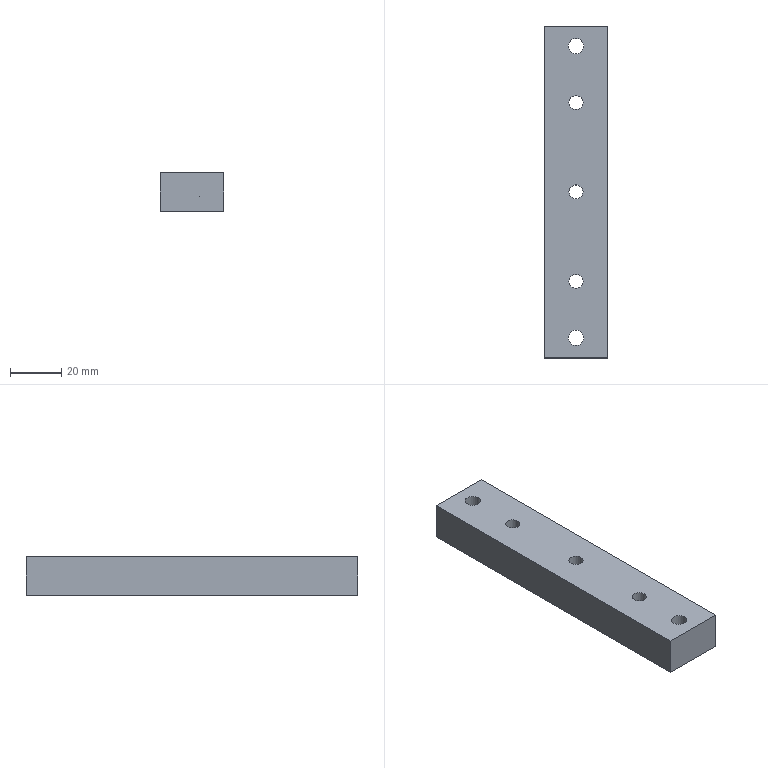Part | STEP file | 200 mesh_id1994 | 1 solid | 11 faces | box 25 x 130 x 15 mm | volume 46833 mm3 | plane 6 | cylinder 5 | commonest cylinder face diameters 5.5 x3 6 x2
STEP:
#1=CARTESIAN_POINT('',(-17225.384,-3957.819,95.));
#2=VERTEX_POINT('',#1);
#3=CARTESIAN_POINT('',(-17225.384,-4087.819,95.));
#4=VERTEX_POINT('',#3);
#5=CARTESIAN_POINT('',(-17225.384,-3961.669,95.));
#6=DIRECTION('',(0.,-1.,0.));
#7=VECTOR('',#6,1.);
#8=LINE('',#5,#7);
#9=EDGE_CURVE('',#2,#4,#8,.T.);
#10=ORIENTED_EDGE('',*,*,#9,.F.);
#11=CARTESIAN_POINT('',(-17225.384,-3957.819,80.));
#12=VERTEX_POINT('',#11);
#13=CARTESIAN_POINT('',(-17225.384,-3957.819,92.));
#14=DIRECTION('',(0.,0.,-1.));
#15=VECTOR('',#14,1.);
#16=LINE('',#13,#15);
#17=EDGE_CURVE('',#2,#12,#16,.T.);
#18=ORIENTED_EDGE('',*,*,#17,.T.);
#19=CARTESIAN_POINT('',(-17225.384,-4087.819,80.));
#20=VERTEX_POINT('',#19);
#21=CARTESIAN_POINT('',(-17225.384,-3961.669,80.));
#22=DIRECTION('',(0.,-1.,0.));
#23=VECTOR('',#22,1.);
#24=LINE('',#21,#23);
#25=EDGE_CURVE('',#12,#20,#24,.T.);
#26=ORIENTED_EDGE('',*,*,#25,.T.);
#27=CARTESIAN_POINT('',(-17225.384,-4087.819,92.));
#28=DIRECTION('',(0.,0.,-1.));
#29=VECTOR('',#28,1.);
#30=LINE('',#27,#29);
#31=EDGE_CURVE('',#4,#20,#30,.T.);
#32=ORIENTED_EDGE('',*,*,#31,.F.);
#33=EDGE_LOOP('',(#10,#18,#26,#32));
#34=FACE_OUTER_BOUND('',#33,.T.);
#35=CARTESIAN_POINT('',(-17225.384,-3961.669,92.));
#36=DIRECTION('',(1.,0.,0.));
#37=DIRECTION('',(0.,0.,1.));
#38=AXIS2_PLACEMENT_3D('',#35,#36,#37);
#39=PLANE('',#38);
#40=ADVANCED_FACE('',(#34),#39,.F.);
#41=CARTESIAN_POINT('',(-17200.384,-4087.819,80.));
#42=VERTEX_POINT('',#41);
#43=CARTESIAN_POINT('',(-17200.384,-3957.819,80.));
#44=VERTEX_POINT('',#43);
#45=CARTESIAN_POINT('',(-17200.384,-4083.969,80.));
#46=DIRECTION('',(0.,1.,0.));
#47=VECTOR('',#46,1.);
#48=LINE('',#45,#47);
#49=EDGE_CURVE('',#42,#44,#48,.T.);
#50=ORIENTED_EDGE('',*,*,#49,.T.);
#51=CARTESIAN_POINT('',(-17200.384,-3957.819,95.));
#52=VERTEX_POINT('',#51);
#53=CARTESIAN_POINT('',(-17200.384,-3957.819,92.));
#54=DIRECTION('',(0.,0.,-1.));
#55=VECTOR('',#54,1.);
#56=LINE('',#53,#55);
#57=EDGE_CURVE('',#52,#44,#56,.T.);
#58=ORIENTED_EDGE('',*,*,#57,.F.);
#59=CARTESIAN_POINT('',(-17200.384,-4087.819,95.));
#60=VERTEX_POINT('',#59);
#61=CARTESIAN_POINT('',(-17200.384,-4083.969,95.));
#62=DIRECTION('',(0.,1.,0.));
#63=VECTOR('',#62,1.);
#64=LINE('',#61,#63);
#65=EDGE_CURVE('',#60,#52,#64,.T.);
#66=ORIENTED_EDGE('',*,*,#65,.F.);
#67=CARTESIAN_POINT('',(-17200.384,-4087.819,92.));
#68=DIRECTION('',(0.,0.,-1.));
#69=VECTOR('',#68,1.);
#70=LINE('',#67,#69);
#71=EDGE_CURVE('',#60,#42,#70,.T.);
#72=ORIENTED_EDGE('',*,*,#71,.T.);
#73=EDGE_LOOP('',(#50,#58,#66,#72));
#74=FACE_OUTER_BOUND('',#73,.T.);
#75=CARTESIAN_POINT('',(-17200.384,-4083.969,92.));
#76=DIRECTION('',(-1.,0.,0.));
#77=DIRECTION('',(0.,0.,-1.));
#78=AXIS2_PLACEMENT_3D('',#75,#76,#77);
#79=PLANE('',#78);
#80=ADVANCED_FACE('',(#74),#79,.F.);
#81=CARTESIAN_POINT('',(-17209.884,-4079.969,95.));
#82=VERTEX_POINT('',#81);
#83=CARTESIAN_POINT('',(-17212.884,-4079.969,95.));
#84=DIRECTION('',(0.,0.,-1.));
#85=DIRECTION('',(1.,0.,0.));
#86=AXIS2_PLACEMENT_3D('',#83,#84,#85);
#87=CIRCLE('',#86,3.);
#88=EDGE_CURVE('',#82,#82,#87,.T.);
#89=ORIENTED_EDGE('',*,*,#88,.T.);
#90=EDGE_LOOP('',(#89));
#91=FACE_BOUND('',#90,.T.);
#92=CARTESIAN_POINT('',(-17209.884,-3965.669,95.));
#93=VERTEX_POINT('',#92);
#94=CARTESIAN_POINT('',(-17212.884,-3965.669,95.));
#95=DIRECTION('',(0.,0.,-1.));
#96=DIRECTION('',(1.,0.,0.));
#97=AXIS2_PLACEMENT_3D('',#94,#95,#96);
#98=CIRCLE('',#97,3.);
#99=EDGE_CURVE('',#93,#93,#98,.T.);
#100=ORIENTED_EDGE('',*,*,#99,.T.);
#101=EDGE_LOOP('',(#100));
#102=FACE_BOUND('',#101,.T.);
#103=ORIENTED_EDGE('',*,*,#65,.T.);
#104=CARTESIAN_POINT('',(-17200.384,-3957.819,95.));
#105=DIRECTION('',(-1.,0.,0.));
#106=VECTOR('',#105,1.);
#107=LINE('',#104,#106);
#108=EDGE_CURVE('',#52,#2,#107,.T.);
#109=ORIENTED_EDGE('',*,*,#108,.T.);
#110=ORIENTED_EDGE('',*,*,#9,.T.);
#111=CARTESIAN_POINT('',(-17225.384,-4087.819,95.));
#112=DIRECTION('',(1.,0.,0.));
#113=VECTOR('',#112,1.);
#114=LINE('',#111,#113);
#115=EDGE_CURVE('',#4,#60,#114,.T.);
#116=ORIENTED_EDGE('',*,*,#115,.T.);
#117=EDGE_LOOP('',(#103,#109,#110,#116));
#118=FACE_BOUND('',#117,.T.);
#119=CARTESIAN_POINT('',(-17210.134,-4057.819,95.));
#120=VERTEX_POINT('',#119);
#121=CARTESIAN_POINT('',(-17212.884,-4057.819,95.));
#122=DIRECTION('',(0.,0.,-1.));
#123=DIRECTION('',(1.,0.,0.));
#124=AXIS2_PLACEMENT_3D('',#121,#122,#123);
#125=CIRCLE('',#124,2.75);
#126=EDGE_CURVE('',#120,#120,#125,.T.);
#127=ORIENTED_EDGE('',*,*,#126,.T.);
#128=EDGE_LOOP('',(#127));
#129=FACE_BOUND('',#128,.T.);
#130=CARTESIAN_POINT('',(-17210.134,-4022.819,95.));
#131=VERTEX_POINT('',#130);
#132=CARTESIAN_POINT('',(-17212.884,-4022.819,95.));
#133=DIRECTION('',(0.,0.,-1.));
#134=DIRECTION('',(1.,0.,0.));
#135=AXIS2_PLACEMENT_3D('',#132,#133,#134);
#136=CIRCLE('',#135,2.75);
#137=EDGE_CURVE('',#131,#131,#136,.T.);
#138=ORIENTED_EDGE('',*,*,#137,.T.);
#139=EDGE_LOOP('',(#138));
#140=FACE_BOUND('',#139,.T.);
#141=CARTESIAN_POINT('',(-17210.134,-3987.819,95.));
#142=VERTEX_POINT('',#141);
#143=CARTESIAN_POINT('',(-17212.884,-3987.819,95.));
#144=DIRECTION('',(0.,0.,-1.));
#145=DIRECTION('',(1.,0.,0.));
#146=AXIS2_PLACEMENT_3D('',#143,#144,#145);
#147=CIRCLE('',#146,2.75);
#148=EDGE_CURVE('',#142,#142,#147,.T.);
#149=ORIENTED_EDGE('',*,*,#148,.T.);
#150=EDGE_LOOP('',(#149));
#151=FACE_BOUND('',#150,.T.);
#152=CARTESIAN_POINT('',(-35.,0.,95.));
#153=DIRECTION('',(0.,0.,1.));
#154=DIRECTION('',(-1.,0.,0.));
#155=AXIS2_PLACEMENT_3D('',#152,#153,#154);
#156=PLANE('',#155);
#157=ADVANCED_FACE('',(#91,#102,#118,#129,#140,#151),#156,.T.);
#158=CARTESIAN_POINT('',(-17215.884,-4079.969,80.));
#159=VERTEX_POINT('',#158);
#160=CARTESIAN_POINT('',(-17212.884,-4079.969,80.));
#161=DIRECTION('',(0.,0.,-1.));
#162=DIRECTION('',(-1.,0.,0.));
#163=AXIS2_PLACEMENT_3D('',#160,#161,#162);
#164=CIRCLE('',#163,3.);
#165=EDGE_CURVE('',#159,#159,#164,.T.);
#166=ORIENTED_EDGE('',*,*,#165,.F.);
#167=EDGE_LOOP('',(#166));
#168=FACE_BOUND('',#167,.T.);
#169=CARTESIAN_POINT('',(-17215.884,-3965.669,80.));
#170=VERTEX_POINT('',#169);
#171=CARTESIAN_POINT('',(-17212.884,-3965.669,80.));
#172=DIRECTION('',(0.,0.,-1.));
#173=DIRECTION('',(-1.,0.,0.));
#174=AXIS2_PLACEMENT_3D('',#171,#172,#173);
#175=CIRCLE('',#174,3.);
#176=EDGE_CURVE('',#170,#170,#175,.T.);
#177=ORIENTED_EDGE('',*,*,#176,.F.);
#178=EDGE_LOOP('',(#177));
#179=FACE_BOUND('',#178,.T.);
#180=CARTESIAN_POINT('',(-17210.134,-4022.819,80.));
#181=VERTEX_POINT('',#180);
#182=CARTESIAN_POINT('',(-17212.884,-4022.819,80.));
#183=DIRECTION('',(0.,0.,1.));
#184=DIRECTION('',(1.,0.,0.));
#185=AXIS2_PLACEMENT_3D('',#182,#183,#184);
#186=CIRCLE('',#185,2.75);
#187=EDGE_CURVE('',#181,#181,#186,.T.);
#188=ORIENTED_EDGE('',*,*,#187,.T.);
#189=EDGE_LOOP('',(#188));
#190=FACE_BOUND('',#189,.T.);
#191=CARTESIAN_POINT('',(-17210.134,-4057.819,80.));
#192=VERTEX_POINT('',#191);
#193=CARTESIAN_POINT('',(-17212.884,-4057.819,80.));
#194=DIRECTION('',(0.,0.,1.));
#195=DIRECTION('',(1.,0.,0.));
#196=AXIS2_PLACEMENT_3D('',#193,#194,#195);
#197=CIRCLE('',#196,2.75);
#198=EDGE_CURVE('',#192,#192,#197,.T.);
#199=ORIENTED_EDGE('',*,*,#198,.T.);
#200=EDGE_LOOP('',(#199));
#201=FACE_BOUND('',#200,.T.);
#202=CARTESIAN_POINT('',(-17200.384,-3957.819,80.));
#203=DIRECTION('',(-1.,0.,0.));
#204=VECTOR('',#203,1.);
#205=LINE('',#202,#204);
#206=EDGE_CURVE('',#44,#12,#205,.T.);
#207=ORIENTED_EDGE('',*,*,#206,.F.);
#208=ORIENTED_EDGE('',*,*,#49,.F.);
#209=CARTESIAN_POINT('',(-17225.384,-4087.819,80.));
#210=DIRECTION('',(1.,0.,0.));
#211=VECTOR('',#210,1.);
#212=LINE('',#209,#211);
#213=EDGE_CURVE('',#20,#42,#212,.T.);
#214=ORIENTED_EDGE('',*,*,#213,.F.);
#215=ORIENTED_EDGE('',*,*,#25,.F.);
#216=EDGE_LOOP('',(#207,#208,#214,#215));
#217=FACE_BOUND('',#216,.T.);
#218=CARTESIAN_POINT('',(-17210.134,-3987.819,80.));
#219=VERTEX_POINT('',#218);
#220=CARTESIAN_POINT('',(-17212.884,-3987.819,80.));
#221=DIRECTION('',(0.,0.,1.));
#222=DIRECTION('',(1.,0.,0.));
#223=AXIS2_PLACEMENT_3D('',#220,#221,#222);
#224=CIRCLE('',#223,2.75);
#225=EDGE_CURVE('',#219,#219,#224,.T.);
#226=ORIENTED_EDGE('',*,*,#225,.T.);
#227=EDGE_LOOP('',(#226));
#228=FACE_BOUND('',#227,.T.);
#229=CARTESIAN_POINT('',(-35.,0.,80.));
#230=DIRECTION('',(0.,0.,1.));
#231=DIRECTION('',(-1.,0.,0.));
#232=AXIS2_PLACEMENT_3D('',#229,#230,#231);
#233=PLANE('',#232);
#234=ADVANCED_FACE('',(#168,#179,#190,#201,#217,#228),#233,.F.);
#235=ORIENTED_EDGE('',*,*,#187,.F.);
#236=EDGE_LOOP('',(#235));
#237=FACE_BOUND('',#236,.T.);
#238=ORIENTED_EDGE('',*,*,#137,.F.);
#239=EDGE_LOOP('',(#238));
#240=FACE_BOUND('',#239,.T.);
#241=CARTESIAN_POINT('',(-17212.884,-4022.819,92.));
#242=DIRECTION('',(0.,0.,-1.));
#243=DIRECTION('',(1.,0.,0.));
#244=AXIS2_PLACEMENT_3D('',#241,#242,#243);
#245=CYLINDRICAL_SURFACE('',#244,2.75);
#246=ADVANCED_FACE('',(#237,#240),#245,.F.);
#247=ORIENTED_EDGE('',*,*,#213,.T.);
#248=ORIENTED_EDGE('',*,*,#71,.F.);
#249=ORIENTED_EDGE('',*,*,#115,.F.);
#250=ORIENTED_EDGE('',*,*,#31,.T.);
#251=EDGE_LOOP('',(#247,#248,#249,#250));
#252=FACE_OUTER_BOUND('',#251,.T.);
#253=CARTESIAN_POINT('',(-17225.384,-4087.819,92.));
#254=DIRECTION('',(0.,1.,0.));
#255=DIRECTION('',(0.,0.,-1.));
#256=AXIS2_PLACEMENT_3D('',#253,#254,#255);
#257=PLANE('',#256);
#258=ADVANCED_FACE('',(#252),#257,.F.);
#259=ORIENTED_EDGE('',*,*,#126,.F.);
#260=EDGE_LOOP('',(#259));
#261=FACE_BOUND('',#260,.T.);
#262=ORIENTED_EDGE('',*,*,#198,.F.);
#263=EDGE_LOOP('',(#262));
#264=FACE_BOUND('',#263,.T.);
#265=CARTESIAN_POINT('',(-17212.884,-4057.819,92.));
#266=DIRECTION('',(0.,0.,-1.));
#267=DIRECTION('',(1.,0.,0.));
#268=AXIS2_PLACEMENT_3D('',#265,#266,#267);
#269=CYLINDRICAL_SURFACE('',#268,2.75);
#270=ADVANCED_FACE('',(#261,#264),#269,.F.);
#271=ORIENTED_EDGE('',*,*,#148,.F.);
#272=EDGE_LOOP('',(#271));
#273=FACE_BOUND('',#272,.T.);
#274=ORIENTED_EDGE('',*,*,#225,.F.);
#275=EDGE_LOOP('',(#274));
#276=FACE_BOUND('',#275,.T.);
#277=CARTESIAN_POINT('',(-17212.884,-3987.819,92.));
#278=DIRECTION('',(0.,0.,-1.));
#279=DIRECTION('',(1.,0.,0.));
#280=AXIS2_PLACEMENT_3D('',#277,#278,#279);
#281=CYLINDRICAL_SURFACE('',#280,2.75);
#282=ADVANCED_FACE('',(#273,#276),#281,.F.);
#283=ORIENTED_EDGE('',*,*,#206,.T.);
#284=ORIENTED_EDGE('',*,*,#17,.F.);
#285=ORIENTED_EDGE('',*,*,#108,.F.);
#286=ORIENTED_EDGE('',*,*,#57,.T.);
#287=EDGE_LOOP('',(#283,#284,#285,#286));
#288=FACE_OUTER_BOUND('',#287,.T.);
#289=CARTESIAN_POINT('',(-17200.384,-3957.819,92.));
#290=DIRECTION('',(0.,-1.,0.));
#291=DIRECTION('',(0.,0.,1.));
#292=AXIS2_PLACEMENT_3D('',#289,#290,#291);
#293=PLANE('',#292);
#294=ADVANCED_FACE('',(#288),#293,.F.);
#295=ORIENTED_EDGE('',*,*,#99,.F.);
#296=EDGE_LOOP('',(#295));
#297=FACE_BOUND('',#296,.T.);
#298=ORIENTED_EDGE('',*,*,#176,.T.);
#299=EDGE_LOOP('',(#298));
#300=FACE_BOUND('',#299,.T.);
#301=CARTESIAN_POINT('',(-17212.884,-3965.669,97.));
#302=DIRECTION('',(0.,0.,-1.));
#303=DIRECTION('',(1.,0.,0.));
#304=AXIS2_PLACEMENT_3D('',#301,#302,#303);
#305=CYLINDRICAL_SURFACE('',#304,3.);
#306=ADVANCED_FACE('',(#297,#300),#305,.F.);
#307=ORIENTED_EDGE('',*,*,#88,.F.);
#308=EDGE_LOOP('',(#307));
#309=FACE_BOUND('',#308,.T.);
#310=ORIENTED_EDGE('',*,*,#165,.T.);
#311=EDGE_LOOP('',(#310));
#312=FACE_BOUND('',#311,.T.);
#313=CARTESIAN_POINT('',(-17212.884,-4079.969,97.));
#314=DIRECTION('',(0.,0.,-1.));
#315=DIRECTION('',(1.,0.,0.));
#316=AXIS2_PLACEMENT_3D('',#313,#314,#315);
#317=CYLINDRICAL_SURFACE('',#316,3.);
#318=ADVANCED_FACE('',(#309,#312),#317,.F.);
#319=CLOSED_SHELL('',(#40,#80,#157,#234,#246,#258,#270,#282,#294,#306,#318));
#320=MANIFOLD_SOLID_BREP('',#319);
#321=(LENGTH_UNIT()NAMED_UNIT(*)SI_UNIT(.MILLI.,.METRE.));
#322=UNCERTAINTY_MEASURE_WITH_UNIT(LENGTH_MEASURE(0.00002),#321,'','');
#323=(NAMED_UNIT(*)PLANE_ANGLE_UNIT()SI_UNIT($,.RADIAN.));
#324=PLANE_ANGLE_MEASURE_WITH_UNIT(PLANE_ANGLE_MEASURE(0.01745),#323);
#325=DIMENSIONAL_EXPONENTS(0.,0.,0.,0.,0.,0.,0.);
#326=(CONVERSION_BASED_UNIT('DEGREE',#324)NAMED_UNIT(#325)PLANE_ANGLE_UNIT());
#327=(NAMED_UNIT(*)SI_UNIT($,.STERADIAN.)SOLID_ANGLE_UNIT());
#328=(GEOMETRIC_REPRESENTATION_CONTEXT(3)GLOBAL_UNCERTAINTY_ASSIGNED_CONTEXT((#322))GLOBAL_UNIT_ASSIGNED_CONTEXT((#321,#326,#327))REPRESENTATION_CONTEXT('',''));
#329=ADVANCED_BREP_SHAPE_REPRESENTATION('',(#320),#328);